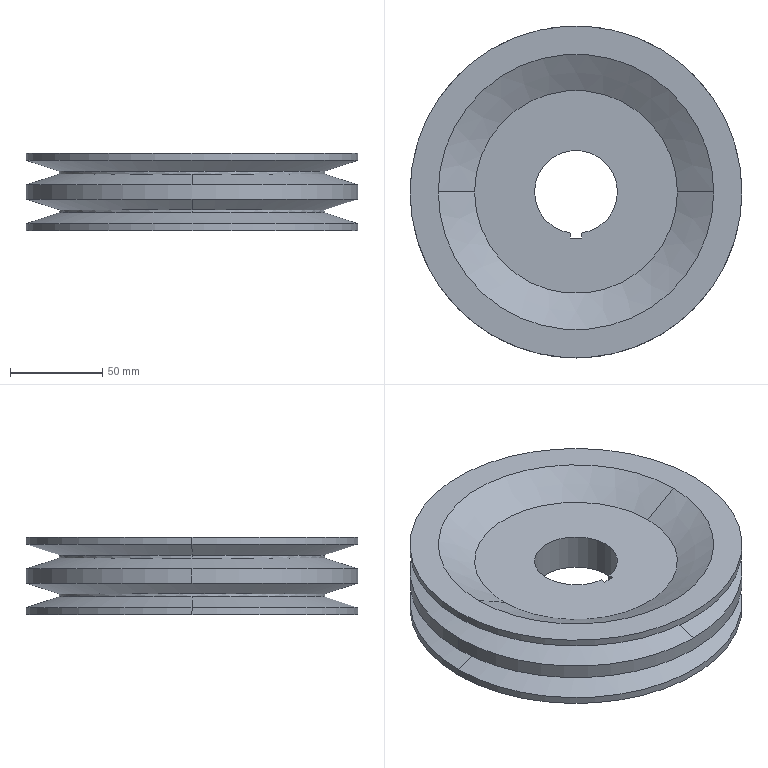Part | SolidWorks | features BaseBody 1 | 1 solid | 30 faces | box 180 x 180 x 42 mm | volume 603331 mm3 | cone 12 | cylinder 11 | plane 7 | commonest cylinder face diameters 180 x6 144 x4 45 x1
STEP:
#1=CARTESIAN_POINT('',(55.,0.,10.));
#2=VERTEX_POINT('',#1);
#3=CARTESIAN_POINT('',(-55.,0.,10.));
#4=VERTEX_POINT('',#3);
#5=CARTESIAN_POINT('',(0.,0.,10.));
#6=DIRECTION('',(0.,0.,-1.));
#7=DIRECTION('',(1.,0.,0.));
#8=AXIS2_PLACEMENT_3D('',#5,#6,#7);
#9=CIRCLE('',#8,55.);
#10=EDGE_CURVE('',#2,#4,#9,.T.);
#11=ORIENTED_EDGE('',*,*,#10,.T.);
#12=CARTESIAN_POINT('',(-74.685,0.,21.));
#13=VERTEX_POINT('',#12);
#14=CARTESIAN_POINT('',(-55.,0.,10.));
#15=DIRECTION('',(-0.873,0.,0.4878));
#16=VECTOR('',#15,1000.);
#17=LINE('',#14,#16);
#18=EDGE_CURVE('',#4,#13,#17,.T.);
#19=ORIENTED_EDGE('',*,*,#18,.T.);
#20=CARTESIAN_POINT('',(74.685,0.,21.));
#21=VERTEX_POINT('',#20);
#22=CARTESIAN_POINT('',(0.,0.,21.));
#23=DIRECTION('',(0.,0.,-1.));
#24=DIRECTION('',(1.,0.,0.));
#25=AXIS2_PLACEMENT_3D('',#22,#23,#24);
#26=CIRCLE('',#25,74.685);
#27=EDGE_CURVE('',#21,#13,#26,.T.);
#28=ORIENTED_EDGE('',*,*,#27,.F.);
#29=CARTESIAN_POINT('',(55.,0.,10.));
#30=DIRECTION('',(0.873,0.,0.4878));
#31=VECTOR('',#30,1000.);
#32=LINE('',#29,#31);
#33=EDGE_CURVE('',#2,#21,#32,.T.);
#34=ORIENTED_EDGE('',*,*,#33,.F.);
#35=EDGE_LOOP('',(#11,#19,#28,#34));
#36=FACE_OUTER_BOUND('',#35,.T.);
#37=CARTESIAN_POINT('',(0.,0.,10.));
#38=DIRECTION('',(0.,0.,1.));
#39=DIRECTION('',(1.,0.,0.));
#40=AXIS2_PLACEMENT_3D('',#37,#38,#39);
#41=CONICAL_SURFACE('',#40,55.,1.061);
#42=ADVANCED_FACE('',(#36),#41,.F.);
#43=CARTESIAN_POINT('',(-55.,0.,-10.));
#44=VERTEX_POINT('',#43);
#45=CARTESIAN_POINT('',(55.,0.,-10.));
#46=VERTEX_POINT('',#45);
#47=CARTESIAN_POINT('',(0.,0.,-10.));
#48=DIRECTION('',(0.,0.,1.));
#49=DIRECTION('',(-1.,0.,0.));
#50=AXIS2_PLACEMENT_3D('',#47,#48,#49);
#51=CIRCLE('',#50,55.);
#52=EDGE_CURVE('',#44,#46,#51,.T.);
#53=ORIENTED_EDGE('',*,*,#52,.T.);
#54=CARTESIAN_POINT('',(74.685,0.,-21.));
#55=VERTEX_POINT('',#54);
#56=CARTESIAN_POINT('',(74.685,0.,-21.));
#57=DIRECTION('',(0.873,0.,-0.4878));
#58=VECTOR('',#57,1000.);
#59=LINE('',#56,#58);
#60=EDGE_CURVE('',#46,#55,#59,.T.);
#61=ORIENTED_EDGE('',*,*,#60,.T.);
#62=CARTESIAN_POINT('',(-74.685,0.,-21.));
#63=VERTEX_POINT('',#62);
#64=CARTESIAN_POINT('',(0.,0.,-21.));
#65=DIRECTION('',(0.,0.,1.));
#66=DIRECTION('',(-1.,0.,0.));
#67=AXIS2_PLACEMENT_3D('',#64,#65,#66);
#68=CIRCLE('',#67,74.685);
#69=EDGE_CURVE('',#63,#55,#68,.T.);
#70=ORIENTED_EDGE('',*,*,#69,.F.);
#71=CARTESIAN_POINT('',(-74.685,0.,-21.));
#72=DIRECTION('',(-0.873,0.,-0.4878));
#73=VECTOR('',#72,1000.);
#74=LINE('',#71,#73);
#75=EDGE_CURVE('',#44,#63,#74,.T.);
#76=ORIENTED_EDGE('',*,*,#75,.F.);
#77=EDGE_LOOP('',(#53,#61,#70,#76));
#78=FACE_OUTER_BOUND('',#77,.T.);
#79=CARTESIAN_POINT('',(0.,0.,-21.));
#80=DIRECTION('',(0.,0.,-1.));
#81=DIRECTION('',(-1.,0.,0.));
#82=AXIS2_PLACEMENT_3D('',#79,#80,#81);
#83=CONICAL_SURFACE('',#82,74.685,1.061);
#84=ADVANCED_FACE('',(#78),#83,.F.);
#85=CARTESIAN_POINT('',(-90.,0.,17.15));
#86=VERTEX_POINT('',#85);
#87=CARTESIAN_POINT('',(90.,0.,17.15));
#88=VERTEX_POINT('',#87);
#89=CARTESIAN_POINT('',(0.,0.,17.15));
#90=DIRECTION('',(0.,0.,-1.));
#91=DIRECTION('',(-1.,0.,0.));
#92=AXIS2_PLACEMENT_3D('',#89,#90,#91);
#93=CIRCLE('',#92,90.);
#94=EDGE_CURVE('',#86,#88,#93,.T.);
#95=ORIENTED_EDGE('',*,*,#94,.F.);
#96=CARTESIAN_POINT('',(-90.,0.,21.));
#97=VERTEX_POINT('',#96);
#98=CARTESIAN_POINT('',(-90.,0.,17.15));
#99=DIRECTION('',(0.,0.,1.));
#100=VECTOR('',#99,1000.);
#101=LINE('',#98,#100);
#102=EDGE_CURVE('',#86,#97,#101,.T.);
#103=ORIENTED_EDGE('',*,*,#102,.T.);
#104=CARTESIAN_POINT('',(90.,0.,21.));
#105=VERTEX_POINT('',#104);
#106=CARTESIAN_POINT('',(0.,0.,21.));
#107=DIRECTION('',(0.,0.,-1.));
#108=DIRECTION('',(1.,0.,0.));
#109=AXIS2_PLACEMENT_3D('',#106,#107,#108);
#110=CIRCLE('',#109,90.);
#111=EDGE_CURVE('',#97,#105,#110,.T.);
#112=ORIENTED_EDGE('',*,*,#111,.T.);
#113=CARTESIAN_POINT('',(90.,0.,17.15));
#114=DIRECTION('',(0.,0.,1.));
#115=VECTOR('',#114,1000.);
#116=LINE('',#113,#115);
#117=EDGE_CURVE('',#88,#105,#116,.T.);
#118=ORIENTED_EDGE('',*,*,#117,.F.);
#119=EDGE_LOOP('',(#95,#103,#112,#118));
#120=FACE_OUTER_BOUND('',#119,.T.);
#121=CARTESIAN_POINT('',(0.,0.,17.15));
#122=DIRECTION('',(0.,0.,1.));
#123=DIRECTION('',(1.,0.,0.));
#124=AXIS2_PLACEMENT_3D('',#121,#122,#123);
#125=CYLINDRICAL_SURFACE('',#124,90.);
#126=ADVANCED_FACE('',(#120),#125,.T.);
#127=CARTESIAN_POINT('',(90.,0.,-21.));
#128=VERTEX_POINT('',#127);
#129=CARTESIAN_POINT('',(-90.,0.,-21.));
#130=VERTEX_POINT('',#129);
#131=CARTESIAN_POINT('',(0.,0.,-21.));
#132=DIRECTION('',(0.,0.,1.));
#133=DIRECTION('',(1.,0.,0.));
#134=AXIS2_PLACEMENT_3D('',#131,#132,#133);
#135=CIRCLE('',#134,90.);
#136=EDGE_CURVE('',#128,#130,#135,.T.);
#137=ORIENTED_EDGE('',*,*,#136,.T.);
#138=CARTESIAN_POINT('',(-90.,0.,-17.15));
#139=VERTEX_POINT('',#138);
#140=CARTESIAN_POINT('',(-90.,0.,-21.));
#141=DIRECTION('',(0.,0.,1.));
#142=VECTOR('',#141,1000.);
#143=LINE('',#140,#142);
#144=EDGE_CURVE('',#130,#139,#143,.T.);
#145=ORIENTED_EDGE('',*,*,#144,.T.);
#146=CARTESIAN_POINT('',(90.,0.,-17.15));
#147=VERTEX_POINT('',#146);
#148=CARTESIAN_POINT('',(0.,0.,-17.15));
#149=DIRECTION('',(0.,0.,1.));
#150=DIRECTION('',(-1.,0.,0.));
#151=AXIS2_PLACEMENT_3D('',#148,#149,#150);
#152=CIRCLE('',#151,90.);
#153=EDGE_CURVE('',#147,#139,#152,.T.);
#154=ORIENTED_EDGE('',*,*,#153,.F.);
#155=CARTESIAN_POINT('',(90.,0.,-21.));
#156=DIRECTION('',(0.,0.,1.));
#157=VECTOR('',#156,1000.);
#158=LINE('',#155,#157);
#159=EDGE_CURVE('',#128,#147,#158,.T.);
#160=ORIENTED_EDGE('',*,*,#159,.F.);
#161=EDGE_LOOP('',(#137,#145,#154,#160));
#162=FACE_OUTER_BOUND('',#161,.T.);
#163=CARTESIAN_POINT('',(0.,0.,-21.));
#164=DIRECTION('',(0.,0.,1.));
#165=DIRECTION('',(1.,0.,0.));
#166=AXIS2_PLACEMENT_3D('',#163,#164,#165);
#167=CYLINDRICAL_SURFACE('',#166,90.);
#168=ADVANCED_FACE('',(#162),#167,.T.);
#169=CARTESIAN_POINT('',(-72.,0.,11.301));
#170=VERTEX_POINT('',#169);
#171=CARTESIAN_POINT('',(72.,0.,11.301));
#172=VERTEX_POINT('',#171);
#173=CARTESIAN_POINT('',(0.,0.,11.301));
#174=DIRECTION('',(0.,0.,-1.));
#175=DIRECTION('',(-1.,0.,0.));
#176=AXIS2_PLACEMENT_3D('',#173,#174,#175);
#177=CIRCLE('',#176,72.);
#178=EDGE_CURVE('',#170,#172,#177,.T.);
#179=ORIENTED_EDGE('',*,*,#178,.F.);
#180=CARTESIAN_POINT('',(-72.,0.,11.301));
#181=DIRECTION('',(-0.9511,0.,0.309));
#182=VECTOR('',#181,1000.);
#183=LINE('',#180,#182);
#184=EDGE_CURVE('',#170,#86,#183,.T.);
#185=ORIENTED_EDGE('',*,*,#184,.T.);
#186=ORIENTED_EDGE('',*,*,#94,.T.);
#187=CARTESIAN_POINT('',(72.,0.,11.301));
#188=DIRECTION('',(0.9511,0.,0.309));
#189=VECTOR('',#188,1000.);
#190=LINE('',#187,#189);
#191=EDGE_CURVE('',#172,#88,#190,.T.);
#192=ORIENTED_EDGE('',*,*,#191,.F.);
#193=EDGE_LOOP('',(#179,#185,#186,#192));
#194=FACE_OUTER_BOUND('',#193,.T.);
#195=CARTESIAN_POINT('',(0.,0.,11.301));
#196=DIRECTION('',(0.,0.,1.));
#197=DIRECTION('',(1.,0.,0.));
#198=AXIS2_PLACEMENT_3D('',#195,#196,#197);
#199=CONICAL_SURFACE('',#198,72.,1.257);
#200=ADVANCED_FACE('',(#194),#199,.T.);
#201=CARTESIAN_POINT('',(72.,0.,-11.301));
#202=VERTEX_POINT('',#201);
#203=CARTESIAN_POINT('',(0.,72.,-11.301));
#204=VERTEX_POINT('',#203);
#205=CARTESIAN_POINT('',(0.,0.,-11.301));
#206=DIRECTION('',(0.,0.,1.));
#207=DIRECTION('',(-1.,0.,0.));
#208=AXIS2_PLACEMENT_3D('',#205,#206,#207);
#209=CIRCLE('',#208,72.);
#210=EDGE_CURVE('',#202,#204,#209,.T.);
#211=ORIENTED_EDGE('',*,*,#210,.F.);
#212=CARTESIAN_POINT('',(90.,0.,-17.15));
#213=DIRECTION('',(0.9511,0.,-0.309));
#214=VECTOR('',#213,1000.);
#215=LINE('',#212,#214);
#216=EDGE_CURVE('',#202,#147,#215,.T.);
#217=ORIENTED_EDGE('',*,*,#216,.T.);
#218=ORIENTED_EDGE('',*,*,#153,.T.);
#219=CARTESIAN_POINT('',(-72.,0.,-11.301));
#220=VERTEX_POINT('',#219);
#221=CARTESIAN_POINT('',(-90.,0.,-17.15));
#222=DIRECTION('',(-0.9511,0.,-0.309));
#223=VECTOR('',#222,1000.);
#224=LINE('',#221,#223);
#225=EDGE_CURVE('',#220,#139,#224,.T.);
#226=ORIENTED_EDGE('',*,*,#225,.F.);
#227=CARTESIAN_POINT('',(0.,0.,-11.301));
#228=DIRECTION('',(0.,0.,1.));
#229=DIRECTION('',(-1.,0.,0.));
#230=AXIS2_PLACEMENT_3D('',#227,#228,#229);
#231=CIRCLE('',#230,72.);
#232=EDGE_CURVE('',#204,#220,#231,.T.);
#233=ORIENTED_EDGE('',*,*,#232,.F.);
#234=EDGE_LOOP('',(#211,#217,#218,#226,#233));
#235=FACE_OUTER_BOUND('',#234,.T.);
#236=CARTESIAN_POINT('',(0.,0.,-17.15));
#237=DIRECTION('',(0.,0.,-1.));
#238=DIRECTION('',(-1.,0.,0.));
#239=AXIS2_PLACEMENT_3D('',#236,#237,#238);
#240=CONICAL_SURFACE('',#239,90.,1.257);
#241=ADVANCED_FACE('',(#235),#240,.T.);
#242=CARTESIAN_POINT('',(-72.,0.,9.699));
#243=VERTEX_POINT('',#242);
#244=CARTESIAN_POINT('',(0.,72.,9.699));
#245=VERTEX_POINT('',#244);
#246=CARTESIAN_POINT('',(0.,0.,9.699));
#247=DIRECTION('',(0.,0.,-1.));
#248=DIRECTION('',(-1.,0.,0.));
#249=AXIS2_PLACEMENT_3D('',#246,#247,#248);
#250=CIRCLE('',#249,72.);
#251=EDGE_CURVE('',#243,#245,#250,.T.);
#252=ORIENTED_EDGE('',*,*,#251,.F.);
#253=CARTESIAN_POINT('',(-72.,0.,9.699));
#254=DIRECTION('',(0.,0.,1.));
#255=VECTOR('',#254,1000.);
#256=LINE('',#253,#255);
#257=EDGE_CURVE('',#243,#170,#256,.T.);
#258=ORIENTED_EDGE('',*,*,#257,.T.);
#259=ORIENTED_EDGE('',*,*,#178,.T.);
#260=CARTESIAN_POINT('',(72.,0.,9.699));
#261=VERTEX_POINT('',#260);
#262=CARTESIAN_POINT('',(72.,0.,9.699));
#263=DIRECTION('',(0.,0.,1.));
#264=VECTOR('',#263,1000.);
#265=LINE('',#262,#264);
#266=EDGE_CURVE('',#261,#172,#265,.T.);
#267=ORIENTED_EDGE('',*,*,#266,.F.);
#268=CARTESIAN_POINT('',(0.,0.,9.699));
#269=DIRECTION('',(0.,0.,-1.));
#270=DIRECTION('',(-1.,0.,0.));
#271=AXIS2_PLACEMENT_3D('',#268,#269,#270);
#272=CIRCLE('',#271,72.);
#273=EDGE_CURVE('',#245,#261,#272,.T.);
#274=ORIENTED_EDGE('',*,*,#273,.F.);
#275=EDGE_LOOP('',(#252,#258,#259,#267,#274));
#276=FACE_OUTER_BOUND('',#275,.T.);
#277=CARTESIAN_POINT('',(0.,0.,9.699));
#278=DIRECTION('',(0.,0.,1.));
#279=DIRECTION('',(1.,0.,0.));
#280=AXIS2_PLACEMENT_3D('',#277,#278,#279);
#281=CYLINDRICAL_SURFACE('',#280,72.);
#282=ADVANCED_FACE('',(#276),#281,.T.);
#283=CARTESIAN_POINT('',(0.,-72.,-11.301));
#284=VERTEX_POINT('',#283);
#285=CARTESIAN_POINT('',(0.,0.,-11.301));
#286=DIRECTION('',(0.,0.,1.));
#287=DIRECTION('',(-1.,0.,0.));
#288=AXIS2_PLACEMENT_3D('',#285,#286,#287);
#289=CIRCLE('',#288,72.);
#290=EDGE_CURVE('',#284,#202,#289,.T.);
#291=ORIENTED_EDGE('',*,*,#290,.T.);
#292=ORIENTED_EDGE('',*,*,#210,.T.);
#293=CARTESIAN_POINT('',(0.,72.,-9.699));
#294=VERTEX_POINT('',#293);
#295=CARTESIAN_POINT('',(0.,72.,-11.301));
#296=DIRECTION('',(0.,0.,1.));
#297=VECTOR('',#296,1000.);
#298=LINE('',#295,#297);
#299=EDGE_CURVE('',#204,#294,#298,.T.);
#300=ORIENTED_EDGE('',*,*,#299,.T.);
#301=CARTESIAN_POINT('',(0.,-72.,-9.699));
#302=VERTEX_POINT('',#301);
#303=CARTESIAN_POINT('',(0.,0.,-9.699));
#304=DIRECTION('',(0.,0.,1.));
#305=DIRECTION('',(-1.,0.,0.));
#306=AXIS2_PLACEMENT_3D('',#303,#304,#305);
#307=CIRCLE('',#306,72.);
#308=EDGE_CURVE('',#302,#294,#307,.T.);
#309=ORIENTED_EDGE('',*,*,#308,.F.);
#310=CARTESIAN_POINT('',(0.,-72.,-11.301));
#311=DIRECTION('',(0.,0.,1.));
#312=VECTOR('',#311,1000.);
#313=LINE('',#310,#312);
#314=EDGE_CURVE('',#284,#302,#313,.T.);
#315=ORIENTED_EDGE('',*,*,#314,.F.);
#316=EDGE_LOOP('',(#291,#292,#300,#309,#315));
#317=FACE_OUTER_BOUND('',#316,.T.);
#318=CARTESIAN_POINT('',(0.,0.,-11.301));
#319=DIRECTION('',(0.,0.,1.));
#320=DIRECTION('',(0.,-1.,0.));
#321=AXIS2_PLACEMENT_3D('',#318,#319,#320);
#322=CYLINDRICAL_SURFACE('',#321,72.);
#323=ADVANCED_FACE('',(#317),#322,.T.);
#324=ORIENTED_EDGE('',*,*,#273,.T.);
#325=CARTESIAN_POINT('',(0.,-72.,9.699));
#326=VERTEX_POINT('',#325);
#327=CARTESIAN_POINT('',(0.,0.,9.699));
#328=DIRECTION('',(0.,0.,-1.));
#329=DIRECTION('',(-1.,0.,0.));
#330=AXIS2_PLACEMENT_3D('',#327,#328,#329);
#331=CIRCLE('',#330,72.);
#332=EDGE_CURVE('',#261,#326,#331,.T.);
#333=ORIENTED_EDGE('',*,*,#332,.T.);
#334=CARTESIAN_POINT('',(0.,-90.,3.85));
#335=VERTEX_POINT('',#334);
#336=CARTESIAN_POINT('',(0.,-90.,3.85));
#337=DIRECTION('',(0.,-0.9511,-0.309));
#338=VECTOR('',#337,1000.);
#339=LINE('',#336,#338);
#340=EDGE_CURVE('',#326,#335,#339,.T.);
#341=ORIENTED_EDGE('',*,*,#340,.T.);
#342=CARTESIAN_POINT('',(90.,0.,3.85));
#343=VERTEX_POINT('',#342);
#344=CARTESIAN_POINT('',(0.,0.,3.85));
#345=DIRECTION('',(0.,0.,-1.));
#346=DIRECTION('',(-1.,0.,0.));
#347=AXIS2_PLACEMENT_3D('',#344,#345,#346);
#348=CIRCLE('',#347,90.);
#349=EDGE_CURVE('',#343,#335,#348,.T.);
#350=ORIENTED_EDGE('',*,*,#349,.F.);
#351=CARTESIAN_POINT('',(0.,90.,3.85));
#352=VERTEX_POINT('',#351);
#353=CARTESIAN_POINT('',(0.,0.,3.85));
#354=DIRECTION('',(0.,0.,-1.));
#355=DIRECTION('',(-1.,0.,0.));
#356=AXIS2_PLACEMENT_3D('',#353,#354,#355);
#357=CIRCLE('',#356,90.);
#358=EDGE_CURVE('',#352,#343,#357,.T.);
#359=ORIENTED_EDGE('',*,*,#358,.F.);
#360=CARTESIAN_POINT('',(0.,90.,3.85));
#361=DIRECTION('',(0.,0.9511,-0.309));
#362=VECTOR('',#361,1000.);
#363=LINE('',#360,#362);
#364=EDGE_CURVE('',#245,#352,#363,.T.);
#365=ORIENTED_EDGE('',*,*,#364,.F.);
#366=EDGE_LOOP('',(#324,#333,#341,#350,#359,#365));
#367=FACE_OUTER_BOUND('',#366,.T.);
#368=CARTESIAN_POINT('',(0.,0.,3.85));
#369=DIRECTION('',(0.,0.,-1.));
#370=DIRECTION('',(0.,1.,0.));
#371=AXIS2_PLACEMENT_3D('',#368,#369,#370);
#372=CONICAL_SURFACE('',#371,90.,1.257);
#373=ADVANCED_FACE('',(#367),#372,.T.);
#374=ORIENTED_EDGE('',*,*,#308,.T.);
#375=CARTESIAN_POINT('',(0.,90.,-3.85));
#376=VERTEX_POINT('',#375);
#377=CARTESIAN_POINT('',(0.,72.,-9.699));
#378=DIRECTION('',(0.,0.9511,0.309));
#379=VECTOR('',#378,1000.);
#380=LINE('',#377,#379);
#381=EDGE_CURVE('',#294,#376,#380,.T.);
#382=ORIENTED_EDGE('',*,*,#381,.T.);
#383=CARTESIAN_POINT('',(90.,0.,-3.85));
#384=VERTEX_POINT('',#383);
#385=CARTESIAN_POINT('',(0.,0.,-3.85));
#386=DIRECTION('',(0.,0.,1.));
#387=DIRECTION('',(-1.,0.,0.));
#388=AXIS2_PLACEMENT_3D('',#385,#386,#387);
#389=CIRCLE('',#388,90.);
#390=EDGE_CURVE('',#384,#376,#389,.T.);
#391=ORIENTED_EDGE('',*,*,#390,.F.);
#392=CARTESIAN_POINT('',(0.,-90.,-3.85));
#393=VERTEX_POINT('',#392);
#394=CARTESIAN_POINT('',(0.,0.,-3.85));
#395=DIRECTION('',(0.,0.,1.));
#396=DIRECTION('',(-1.,0.,0.));
#397=AXIS2_PLACEMENT_3D('',#394,#395,#396);
#398=CIRCLE('',#397,90.);
#399=EDGE_CURVE('',#393,#384,#398,.T.);
#400=ORIENTED_EDGE('',*,*,#399,.F.);
#401=CARTESIAN_POINT('',(0.,-72.,-9.699));
#402=DIRECTION('',(0.,-0.9511,0.309));
#403=VECTOR('',#402,1000.);
#404=LINE('',#401,#403);
#405=EDGE_CURVE('',#302,#393,#404,.T.);
#406=ORIENTED_EDGE('',*,*,#405,.F.);
#407=EDGE_LOOP('',(#374,#382,#391,#400,#406));
#408=FACE_OUTER_BOUND('',#407,.T.);
#409=CARTESIAN_POINT('',(0.,0.,-9.699));
#410=DIRECTION('',(0.,0.,1.));
#411=DIRECTION('',(0.,-1.,0.));
#412=AXIS2_PLACEMENT_3D('',#409,#410,#411);
#413=CONICAL_SURFACE('',#412,72.,1.257);
#414=ADVANCED_FACE('',(#408),#413,.T.);
#415=ORIENTED_EDGE('',*,*,#390,.T.);
#416=CARTESIAN_POINT('',(-90.,0.,-3.85));
#417=VERTEX_POINT('',#416);
#418=CARTESIAN_POINT('',(0.,0.,-3.85));
#419=DIRECTION('',(0.,0.,1.));
#420=DIRECTION('',(-1.,0.,0.));
#421=AXIS2_PLACEMENT_3D('',#418,#419,#420);
#422=CIRCLE('',#421,90.);
#423=EDGE_CURVE('',#376,#417,#422,.T.);
#424=ORIENTED_EDGE('',*,*,#423,.T.);
#425=CARTESIAN_POINT('',(-90.,0.,3.85));
#426=VERTEX_POINT('',#425);
#427=CARTESIAN_POINT('',(-90.,0.,-3.85));
#428=DIRECTION('',(0.,0.,1.));
#429=VECTOR('',#428,1000.);
#430=LINE('',#427,#429);
#431=EDGE_CURVE('',#417,#426,#430,.T.);
#432=ORIENTED_EDGE('',*,*,#431,.T.);
#433=CARTESIAN_POINT('',(0.,0.,3.85));
#434=DIRECTION('',(0.,0.,-1.));
#435=DIRECTION('',(-1.,0.,0.));
#436=AXIS2_PLACEMENT_3D('',#433,#434,#435);
#437=CIRCLE('',#436,90.);
#438=EDGE_CURVE('',#426,#352,#437,.T.);
#439=ORIENTED_EDGE('',*,*,#438,.T.);
#440=ORIENTED_EDGE('',*,*,#358,.T.);
#441=CARTESIAN_POINT('',(90.,0.,-3.85));
#442=DIRECTION('',(0.,0.,1.));
#443=VECTOR('',#442,1000.);
#444=LINE('',#441,#443);
#445=EDGE_CURVE('',#384,#343,#444,.T.);
#446=ORIENTED_EDGE('',*,*,#445,.F.);
#447=EDGE_LOOP('',(#415,#424,#432,#439,#440,#446));
#448=FACE_OUTER_BOUND('',#447,.T.);
#449=CARTESIAN_POINT('',(0.,0.,-3.85));
#450=DIRECTION('',(0.,0.,1.));
#451=DIRECTION('',(1.,0.,0.));
#452=AXIS2_PLACEMENT_3D('',#449,#450,#451);
#453=CYLINDRICAL_SURFACE('',#452,90.);
#454=ADVANCED_FACE('',(#448),#453,.T.);
#455=CARTESIAN_POINT('',(-3.,-22.299,10.));
#456=VERTEX_POINT('',#455);
#457=CARTESIAN_POINT('',(3.,-22.299,10.));
#458=VERTEX_POINT('',#457);
#459=CARTESIAN_POINT('',(0.,0.,10.));
#460=DIRECTION('',(0.,0.,-1.));
#461=DIRECTION('',(0.,-1.,0.));
#462=AXIS2_PLACEMENT_3D('',#459,#460,#461);
#463=CIRCLE('',#462,22.5);
#464=EDGE_CURVE('',#456,#458,#463,.T.);
#465=ORIENTED_EDGE('',*,*,#464,.F.);
#466=CARTESIAN_POINT('',(-3.,-22.299,-10.));
#467=VERTEX_POINT('',#466);
#468=CARTESIAN_POINT('',(-3.,-22.299,0.));
#469=DIRECTION('',(0.,0.,1.));
#470=VECTOR('',#469,1000.);
#471=LINE('',#468,#470);
#472=EDGE_CURVE('',#467,#456,#471,.T.);
#473=ORIENTED_EDGE('',*,*,#472,.F.);
#474=CARTESIAN_POINT('',(3.,-22.299,-10.));
#475=VERTEX_POINT('',#474);
#476=CARTESIAN_POINT('',(0.,0.,-10.));
#477=DIRECTION('',(0.,0.,1.));
#478=DIRECTION('',(0.,-1.,0.));
#479=AXIS2_PLACEMENT_3D('',#476,#477,#478);
#480=CIRCLE('',#479,22.5);
#481=EDGE_CURVE('',#475,#467,#480,.T.);
#482=ORIENTED_EDGE('',*,*,#481,.F.);
#483=CARTESIAN_POINT('',(3.,-22.299,0.));
#484=DIRECTION('',(0.,0.,-1.));
#485=VECTOR('',#484,1000.);
#486=LINE('',#483,#485);
#487=EDGE_CURVE('',#458,#475,#486,.T.);
#488=ORIENTED_EDGE('',*,*,#487,.F.);
#489=EDGE_LOOP('',(#465,#473,#482,#488));
#490=FACE_OUTER_BOUND('',#489,.T.);
#491=CARTESIAN_POINT('',(0.,0.,-10.));
#492=DIRECTION('',(0.,0.,1.));
#493=DIRECTION('',(0.,-1.,0.));
#494=AXIS2_PLACEMENT_3D('',#491,#492,#493);
#495=CYLINDRICAL_SURFACE('',#494,22.5);
#496=ADVANCED_FACE('',(#490),#495,.F.);
#497=CARTESIAN_POINT('',(3.,-25.,-10.));
#498=VERTEX_POINT('',#497);
#499=CARTESIAN_POINT('',(3.,-23.65,-10.));
#500=DIRECTION('',(0.,1.,0.));
#501=VECTOR('',#500,1000.);
#502=LINE('',#499,#501);
#503=EDGE_CURVE('',#498,#475,#502,.T.);
#504=ORIENTED_EDGE('',*,*,#503,.F.);
#505=CARTESIAN_POINT('',(3.,-25.,10.));
#506=VERTEX_POINT('',#505);
#507=CARTESIAN_POINT('',(3.,-25.,0.));
#508=DIRECTION('',(0.,0.,-1.));
#509=VECTOR('',#508,1000.);
#510=LINE('',#507,#509);
#511=EDGE_CURVE('',#506,#498,#510,.T.);
#512=ORIENTED_EDGE('',*,*,#511,.F.);
#513=CARTESIAN_POINT('',(3.,-23.65,10.));
#514=DIRECTION('',(0.,-1.,0.));
#515=VECTOR('',#514,1000.);
#516=LINE('',#513,#515);
#517=EDGE_CURVE('',#458,#506,#516,.T.);
#518=ORIENTED_EDGE('',*,*,#517,.F.);
#519=ORIENTED_EDGE('',*,*,#487,.T.);
#520=EDGE_LOOP('',(#504,#512,#518,#519));
#521=FACE_OUTER_BOUND('',#520,.T.);
#522=CARTESIAN_POINT('',(3.,-25.31,-10.4));
#523=DIRECTION('',(1.,0.,0.));
#524=DIRECTION('',(0.,1.,0.));
#525=AXIS2_PLACEMENT_3D('',#522,#523,#524);
#526=PLANE('',#525);
#527=ADVANCED_FACE('',(#521),#526,.F.);
#528=CARTESIAN_POINT('',(-3.,-25.,10.));
#529=VERTEX_POINT('',#528);
#530=CARTESIAN_POINT('',(0.,-25.,10.));
#531=DIRECTION('',(1.,0.,0.));
#532=VECTOR('',#531,1000.);
#533=LINE('',#530,#532);
#534=EDGE_CURVE('',#529,#506,#533,.T.);
#535=ORIENTED_EDGE('',*,*,#534,.F.);
#536=CARTESIAN_POINT('',(-3.,0.,10.));
#537=DIRECTION('',(0.,-1.,0.));
#538=VECTOR('',#537,1000.);
#539=LINE('',#536,#538);
#540=EDGE_CURVE('',#456,#529,#539,.T.);
#541=ORIENTED_EDGE('',*,*,#540,.F.);
#542=ORIENTED_EDGE('',*,*,#464,.T.);
#543=ORIENTED_EDGE('',*,*,#517,.T.);
#544=EDGE_LOOP('',(#535,#541,#542,#543));
#545=FACE_BOUND('',#544,.T.);
#546=ORIENTED_EDGE('',*,*,#10,.F.);
#547=CARTESIAN_POINT('',(0.,0.,10.));
#548=DIRECTION('',(0.,0.,-1.));
#549=DIRECTION('',(1.,0.,0.));
#550=AXIS2_PLACEMENT_3D('',#547,#548,#549);
#551=CIRCLE('',#550,55.);
#552=EDGE_CURVE('',#4,#2,#551,.T.);
#553=ORIENTED_EDGE('',*,*,#552,.F.);
#554=EDGE_LOOP('',(#546,#553));
#555=FACE_OUTER_BOUND('',#554,.T.);
#556=CARTESIAN_POINT('',(57.2,57.2,10.));
#557=DIRECTION('',(0.,0.,1.));
#558=DIRECTION('',(-1.,0.,0.));
#559=AXIS2_PLACEMENT_3D('',#556,#557,#558);
#560=PLANE('',#559);
#561=ADVANCED_FACE('',(#545,#555),#560,.T.);
#562=CARTESIAN_POINT('',(-3.,-25.,-10.));
#563=VERTEX_POINT('',#562);
#564=CARTESIAN_POINT('',(-3.,-23.65,-10.));
#565=DIRECTION('',(0.,-1.,0.));
#566=VECTOR('',#565,1000.);
#567=LINE('',#564,#566);
#568=EDGE_CURVE('',#467,#563,#567,.T.);
#569=ORIENTED_EDGE('',*,*,#568,.F.);
#570=ORIENTED_EDGE('',*,*,#472,.T.);
#571=ORIENTED_EDGE('',*,*,#540,.T.);
#572=CARTESIAN_POINT('',(-3.,-25.,0.));
#573=DIRECTION('',(0.,0.,1.));
#574=VECTOR('',#573,1000.);
#575=LINE('',#572,#574);
#576=EDGE_CURVE('',#563,#529,#575,.T.);
#577=ORIENTED_EDGE('',*,*,#576,.F.);
#578=EDGE_LOOP('',(#569,#570,#571,#577));
#579=FACE_OUTER_BOUND('',#578,.T.);
#580=CARTESIAN_POINT('',(-3.,-21.989,-10.4));
#581=DIRECTION('',(-1.,0.,0.));
#582=DIRECTION('',(0.,-1.,0.));
#583=AXIS2_PLACEMENT_3D('',#580,#581,#582);
#584=PLANE('',#583);
#585=ADVANCED_FACE('',(#579),#584,.F.);
#586=CARTESIAN_POINT('',(0.,-25.,-10.));
#587=DIRECTION('',(-1.,0.,0.));
#588=VECTOR('',#587,1000.);
#589=LINE('',#586,#588);
#590=EDGE_CURVE('',#498,#563,#589,.T.);
#591=ORIENTED_EDGE('',*,*,#590,.F.);
#592=ORIENTED_EDGE('',*,*,#503,.T.);
#593=ORIENTED_EDGE('',*,*,#481,.T.);
#594=ORIENTED_EDGE('',*,*,#568,.T.);
#595=EDGE_LOOP('',(#591,#592,#593,#594));
#596=FACE_BOUND('',#595,.T.);
#597=ORIENTED_EDGE('',*,*,#52,.F.);
#598=CARTESIAN_POINT('',(0.,0.,-10.));
#599=DIRECTION('',(0.,0.,1.));
#600=DIRECTION('',(-1.,0.,0.));
#601=AXIS2_PLACEMENT_3D('',#598,#599,#600);
#602=CIRCLE('',#601,55.);
#603=EDGE_CURVE('',#46,#44,#602,.T.);
#604=ORIENTED_EDGE('',*,*,#603,.F.);
#605=EDGE_LOOP('',(#597,#604));
#606=FACE_OUTER_BOUND('',#605,.T.);
#607=CARTESIAN_POINT('',(57.2,57.2,-10.));
#608=DIRECTION('',(0.,0.,1.));
#609=DIRECTION('',(-1.,0.,0.));
#610=AXIS2_PLACEMENT_3D('',#607,#608,#609);
#611=PLANE('',#610);
#612=ADVANCED_FACE('',(#596,#606),#611,.F.);
#613=ORIENTED_EDGE('',*,*,#590,.T.);
#614=ORIENTED_EDGE('',*,*,#576,.T.);
#615=ORIENTED_EDGE('',*,*,#534,.T.);
#616=ORIENTED_EDGE('',*,*,#511,.T.);
#617=EDGE_LOOP('',(#613,#614,#615,#616));
#618=FACE_OUTER_BOUND('',#617,.T.);
#619=CARTESIAN_POINT('',(-3.31,-25.,-10.4));
#620=DIRECTION('',(0.,-1.,0.));
#621=DIRECTION('',(1.,0.,0.));
#622=AXIS2_PLACEMENT_3D('',#619,#620,#621);
#623=PLANE('',#622);
#624=ADVANCED_FACE('',(#618),#623,.F.);
#625=ORIENTED_EDGE('',*,*,#18,.F.);
#626=ORIENTED_EDGE('',*,*,#552,.T.);
#627=ORIENTED_EDGE('',*,*,#33,.T.);
#628=CARTESIAN_POINT('',(0.,0.,21.));
#629=DIRECTION('',(0.,0.,-1.));
#630=DIRECTION('',(1.,0.,0.));
#631=AXIS2_PLACEMENT_3D('',#628,#629,#630);
#632=CIRCLE('',#631,74.685);
#633=EDGE_CURVE('',#13,#21,#632,.T.);
#634=ORIENTED_EDGE('',*,*,#633,.F.);
#635=EDGE_LOOP('',(#625,#626,#627,#634));
#636=FACE_OUTER_BOUND('',#635,.T.);
#637=CARTESIAN_POINT('',(0.,0.,10.));
#638=DIRECTION('',(0.,0.,1.));
#639=DIRECTION('',(1.,0.,0.));
#640=AXIS2_PLACEMENT_3D('',#637,#638,#639);
#641=CONICAL_SURFACE('',#640,55.,1.061);
#642=ADVANCED_FACE('',(#636),#641,.F.);
#643=ORIENTED_EDGE('',*,*,#60,.F.);
#644=ORIENTED_EDGE('',*,*,#603,.T.);
#645=ORIENTED_EDGE('',*,*,#75,.T.);
#646=CARTESIAN_POINT('',(0.,0.,-21.));
#647=DIRECTION('',(0.,0.,1.));
#648=DIRECTION('',(-1.,0.,0.));
#649=AXIS2_PLACEMENT_3D('',#646,#647,#648);
#650=CIRCLE('',#649,74.685);
#651=EDGE_CURVE('',#55,#63,#650,.T.);
#652=ORIENTED_EDGE('',*,*,#651,.F.);
#653=EDGE_LOOP('',(#643,#644,#645,#652));
#654=FACE_OUTER_BOUND('',#653,.T.);
#655=CARTESIAN_POINT('',(0.,0.,-21.));
#656=DIRECTION('',(0.,0.,-1.));
#657=DIRECTION('',(-1.,0.,0.));
#658=AXIS2_PLACEMENT_3D('',#655,#656,#657);
#659=CONICAL_SURFACE('',#658,74.685,1.061);
#660=ADVANCED_FACE('',(#654),#659,.F.);
#661=ORIENTED_EDGE('',*,*,#27,.T.);
#662=ORIENTED_EDGE('',*,*,#633,.T.);
#663=EDGE_LOOP('',(#661,#662));
#664=FACE_BOUND('',#663,.T.);
#665=CARTESIAN_POINT('',(0.,0.,21.));
#666=DIRECTION('',(0.,0.,-1.));
#667=DIRECTION('',(1.,0.,0.));
#668=AXIS2_PLACEMENT_3D('',#665,#666,#667);
#669=CIRCLE('',#668,90.);
#670=EDGE_CURVE('',#105,#97,#669,.T.);
#671=ORIENTED_EDGE('',*,*,#670,.F.);
#672=ORIENTED_EDGE('',*,*,#111,.F.);
#673=EDGE_LOOP('',(#671,#672));
#674=FACE_OUTER_BOUND('',#673,.T.);
#675=CARTESIAN_POINT('',(93.6,93.632,21.));
#676=DIRECTION('',(0.,0.,1.));
#677=DIRECTION('',(-1.,0.,0.));
#678=AXIS2_PLACEMENT_3D('',#675,#676,#677);
#679=PLANE('',#678);
#680=ADVANCED_FACE('',(#664,#674),#679,.T.);
#681=ORIENTED_EDGE('',*,*,#69,.T.);
#682=ORIENTED_EDGE('',*,*,#651,.T.);
#683=EDGE_LOOP('',(#681,#682));
#684=FACE_BOUND('',#683,.T.);
#685=ORIENTED_EDGE('',*,*,#136,.F.);
#686=CARTESIAN_POINT('',(0.,0.,-21.));
#687=DIRECTION('',(0.,0.,1.));
#688=DIRECTION('',(1.,0.,0.));
#689=AXIS2_PLACEMENT_3D('',#686,#687,#688);
#690=CIRCLE('',#689,90.);
#691=EDGE_CURVE('',#130,#128,#690,.T.);
#692=ORIENTED_EDGE('',*,*,#691,.F.);
#693=EDGE_LOOP('',(#685,#692));
#694=FACE_OUTER_BOUND('',#693,.T.);
#695=CARTESIAN_POINT('',(93.6,93.632,-21.));
#696=DIRECTION('',(0.,0.,1.));
#697=DIRECTION('',(-1.,0.,0.));
#698=AXIS2_PLACEMENT_3D('',#695,#696,#697);
#699=PLANE('',#698);
#700=ADVANCED_FACE('',(#684,#694),#699,.F.);
#701=ORIENTED_EDGE('',*,*,#102,.F.);
#702=CARTESIAN_POINT('',(0.,0.,17.15));
#703=DIRECTION('',(0.,0.,-1.));
#704=DIRECTION('',(-1.,0.,0.));
#705=AXIS2_PLACEMENT_3D('',#702,#703,#704);
#706=CIRCLE('',#705,90.);
#707=EDGE_CURVE('',#88,#86,#706,.T.);
#708=ORIENTED_EDGE('',*,*,#707,.F.);
#709=ORIENTED_EDGE('',*,*,#117,.T.);
#710=ORIENTED_EDGE('',*,*,#670,.T.);
#711=EDGE_LOOP('',(#701,#708,#709,#710));
#712=FACE_OUTER_BOUND('',#711,.T.);
#713=CARTESIAN_POINT('',(0.,0.,17.15));
#714=DIRECTION('',(0.,0.,1.));
#715=DIRECTION('',(1.,0.,0.));
#716=AXIS2_PLACEMENT_3D('',#713,#714,#715);
#717=CYLINDRICAL_SURFACE('',#716,90.);
#718=ADVANCED_FACE('',(#712),#717,.T.);
#719=ORIENTED_EDGE('',*,*,#144,.F.);
#720=ORIENTED_EDGE('',*,*,#691,.T.);
#721=ORIENTED_EDGE('',*,*,#159,.T.);
#722=CARTESIAN_POINT('',(0.,0.,-17.15));
#723=DIRECTION('',(0.,0.,1.));
#724=DIRECTION('',(-1.,0.,0.));
#725=AXIS2_PLACEMENT_3D('',#722,#723,#724);
#726=CIRCLE('',#725,90.);
#727=EDGE_CURVE('',#139,#147,#726,.T.);
#728=ORIENTED_EDGE('',*,*,#727,.F.);
#729=EDGE_LOOP('',(#719,#720,#721,#728));
#730=FACE_OUTER_BOUND('',#729,.T.);
#731=CARTESIAN_POINT('',(0.,0.,-21.));
#732=DIRECTION('',(0.,0.,1.));
#733=DIRECTION('',(1.,0.,0.));
#734=AXIS2_PLACEMENT_3D('',#731,#732,#733);
#735=CYLINDRICAL_SURFACE('',#734,90.);
#736=ADVANCED_FACE('',(#730),#735,.T.);
#737=ORIENTED_EDGE('',*,*,#184,.F.);
#738=CARTESIAN_POINT('',(0.,0.,11.301));
#739=DIRECTION('',(0.,0.,-1.));
#740=DIRECTION('',(-1.,0.,0.));
#741=AXIS2_PLACEMENT_3D('',#738,#739,#740);
#742=CIRCLE('',#741,72.);
#743=EDGE_CURVE('',#172,#170,#742,.T.);
#744=ORIENTED_EDGE('',*,*,#743,.F.);
#745=ORIENTED_EDGE('',*,*,#191,.T.);
#746=ORIENTED_EDGE('',*,*,#707,.T.);
#747=EDGE_LOOP('',(#737,#744,#745,#746));
#748=FACE_OUTER_BOUND('',#747,.T.);
#749=CARTESIAN_POINT('',(0.,0.,11.301));
#750=DIRECTION('',(0.,0.,1.));
#751=DIRECTION('',(1.,0.,0.));
#752=AXIS2_PLACEMENT_3D('',#749,#750,#751);
#753=CONICAL_SURFACE('',#752,72.,1.257);
#754=ADVANCED_FACE('',(#748),#753,.T.);
#755=ORIENTED_EDGE('',*,*,#216,.F.);
#756=ORIENTED_EDGE('',*,*,#290,.F.);
#757=CARTESIAN_POINT('',(0.,0.,-11.301));
#758=DIRECTION('',(0.,0.,1.));
#759=DIRECTION('',(-1.,0.,0.));
#760=AXIS2_PLACEMENT_3D('',#757,#758,#759);
#761=CIRCLE('',#760,72.);
#762=EDGE_CURVE('',#220,#284,#761,.T.);
#763=ORIENTED_EDGE('',*,*,#762,.F.);
#764=ORIENTED_EDGE('',*,*,#225,.T.);
#765=ORIENTED_EDGE('',*,*,#727,.T.);
#766=EDGE_LOOP('',(#755,#756,#763,#764,#765));
#767=FACE_OUTER_BOUND('',#766,.T.);
#768=CARTESIAN_POINT('',(0.,0.,-17.15));
#769=DIRECTION('',(0.,0.,-1.));
#770=DIRECTION('',(-1.,0.,0.));
#771=AXIS2_PLACEMENT_3D('',#768,#769,#770);
#772=CONICAL_SURFACE('',#771,90.,1.257);
#773=ADVANCED_FACE('',(#767),#772,.T.);
#774=ORIENTED_EDGE('',*,*,#257,.F.);
#775=CARTESIAN_POINT('',(0.,0.,9.699));
#776=DIRECTION('',(0.,0.,-1.));
#777=DIRECTION('',(-1.,0.,0.));
#778=AXIS2_PLACEMENT_3D('',#775,#776,#777);
#779=CIRCLE('',#778,72.);
#780=EDGE_CURVE('',#326,#243,#779,.T.);
#781=ORIENTED_EDGE('',*,*,#780,.F.);
#782=ORIENTED_EDGE('',*,*,#332,.F.);
#783=ORIENTED_EDGE('',*,*,#266,.T.);
#784=ORIENTED_EDGE('',*,*,#743,.T.);
#785=EDGE_LOOP('',(#774,#781,#782,#783,#784));
#786=FACE_OUTER_BOUND('',#785,.T.);
#787=CARTESIAN_POINT('',(0.,0.,9.699));
#788=DIRECTION('',(0.,0.,1.));
#789=DIRECTION('',(1.,0.,0.));
#790=AXIS2_PLACEMENT_3D('',#787,#788,#789);
#791=CYLINDRICAL_SURFACE('',#790,72.);
#792=ADVANCED_FACE('',(#786),#791,.T.);
#793=ORIENTED_EDGE('',*,*,#299,.F.);
#794=ORIENTED_EDGE('',*,*,#232,.T.);
#795=ORIENTED_EDGE('',*,*,#762,.T.);
#796=ORIENTED_EDGE('',*,*,#314,.T.);
#797=CARTESIAN_POINT('',(0.,0.,-9.699));
#798=DIRECTION('',(0.,0.,1.));
#799=DIRECTION('',(-1.,0.,0.));
#800=AXIS2_PLACEMENT_3D('',#797,#798,#799);
#801=CIRCLE('',#800,72.);
#802=EDGE_CURVE('',#294,#302,#801,.T.);
#803=ORIENTED_EDGE('',*,*,#802,.F.);
#804=EDGE_LOOP('',(#793,#794,#795,#796,#803));
#805=FACE_OUTER_BOUND('',#804,.T.);
#806=CARTESIAN_POINT('',(0.,0.,-11.301));
#807=DIRECTION('',(0.,0.,1.));
#808=DIRECTION('',(0.,-1.,0.));
#809=AXIS2_PLACEMENT_3D('',#806,#807,#808);
#810=CYLINDRICAL_SURFACE('',#809,72.);
#811=ADVANCED_FACE('',(#805),#810,.T.);
#812=ORIENTED_EDGE('',*,*,#340,.F.);
#813=ORIENTED_EDGE('',*,*,#780,.T.);
#814=ORIENTED_EDGE('',*,*,#251,.T.);
#815=ORIENTED_EDGE('',*,*,#364,.T.);
#816=ORIENTED_EDGE('',*,*,#438,.F.);
#817=CARTESIAN_POINT('',(0.,0.,3.85));
#818=DIRECTION('',(0.,0.,-1.));
#819=DIRECTION('',(-1.,0.,0.));
#820=AXIS2_PLACEMENT_3D('',#817,#818,#819);
#821=CIRCLE('',#820,90.);
#822=EDGE_CURVE('',#335,#426,#821,.T.);
#823=ORIENTED_EDGE('',*,*,#822,.F.);
#824=EDGE_LOOP('',(#812,#813,#814,#815,#816,#823));
#825=FACE_OUTER_BOUND('',#824,.T.);
#826=CARTESIAN_POINT('',(0.,0.,3.85));
#827=DIRECTION('',(0.,0.,-1.));
#828=DIRECTION('',(0.,1.,0.));
#829=AXIS2_PLACEMENT_3D('',#826,#827,#828);
#830=CONICAL_SURFACE('',#829,90.,1.257);
#831=ADVANCED_FACE('',(#825),#830,.T.);
#832=ORIENTED_EDGE('',*,*,#381,.F.);
#833=ORIENTED_EDGE('',*,*,#802,.T.);
#834=ORIENTED_EDGE('',*,*,#405,.T.);
#835=CARTESIAN_POINT('',(0.,0.,-3.85));
#836=DIRECTION('',(0.,0.,1.));
#837=DIRECTION('',(-1.,0.,0.));
#838=AXIS2_PLACEMENT_3D('',#835,#836,#837);
#839=CIRCLE('',#838,90.);
#840=EDGE_CURVE('',#417,#393,#839,.T.);
#841=ORIENTED_EDGE('',*,*,#840,.F.);
#842=ORIENTED_EDGE('',*,*,#423,.F.);
#843=EDGE_LOOP('',(#832,#833,#834,#841,#842));
#844=FACE_OUTER_BOUND('',#843,.T.);
#845=CARTESIAN_POINT('',(0.,0.,-9.699));
#846=DIRECTION('',(0.,0.,1.));
#847=DIRECTION('',(0.,-1.,0.));
#848=AXIS2_PLACEMENT_3D('',#845,#846,#847);
#849=CONICAL_SURFACE('',#848,72.,1.257);
#850=ADVANCED_FACE('',(#844),#849,.T.);
#851=ORIENTED_EDGE('',*,*,#431,.F.);
#852=ORIENTED_EDGE('',*,*,#840,.T.);
#853=ORIENTED_EDGE('',*,*,#399,.T.);
#854=ORIENTED_EDGE('',*,*,#445,.T.);
#855=ORIENTED_EDGE('',*,*,#349,.T.);
#856=ORIENTED_EDGE('',*,*,#822,.T.);
#857=EDGE_LOOP('',(#851,#852,#853,#854,#855,#856));
#858=FACE_OUTER_BOUND('',#857,.T.);
#859=CARTESIAN_POINT('',(0.,0.,-3.85));
#860=DIRECTION('',(0.,0.,1.));
#861=DIRECTION('',(1.,0.,0.));
#862=AXIS2_PLACEMENT_3D('',#859,#860,#861);
#863=CYLINDRICAL_SURFACE('',#862,90.);
#864=ADVANCED_FACE('',(#858),#863,.T.);
#865=CLOSED_SHELL('',(#42,#84,#126,#168,#200,#241,#282,#323,#373,#414,#454,#496,#527,#561,#585,#612,#624,#642,#660,#680,#700,#718,#736,#754,#773,#792,#811,#831,#850,#864));
#866=MANIFOLD_SOLID_BREP('',#865);
#867=CARTESIAN_POINT('',(0.,0.,0.));
#868=DIRECTION('',(0.,0.,1.));
#869=DIRECTION('',(1.,0.,0.));
#870=AXIS2_PLACEMENT_3D('',#867,#868,#869);
#871=(LENGTH_UNIT()NAMED_UNIT(*)SI_UNIT(.MILLI.,.METRE.));
#872=UNCERTAINTY_MEASURE_WITH_UNIT(LENGTH_MEASURE(0.00001),#871,'','');
#873=(NAMED_UNIT(*)PLANE_ANGLE_UNIT()SI_UNIT($,.RADIAN.));
#874=(NAMED_UNIT(*)SI_UNIT($,.STERADIAN.)SOLID_ANGLE_UNIT());
#875=(GEOMETRIC_REPRESENTATION_CONTEXT(3)GLOBAL_UNCERTAINTY_ASSIGNED_CONTEXT((#872))GLOBAL_UNIT_ASSIGNED_CONTEXT((#871,#873,#874))REPRESENTATION_CONTEXT('',''));
#876=ADVANCED_BREP_SHAPE_REPRESENTATION('',(#866,#870),#875);